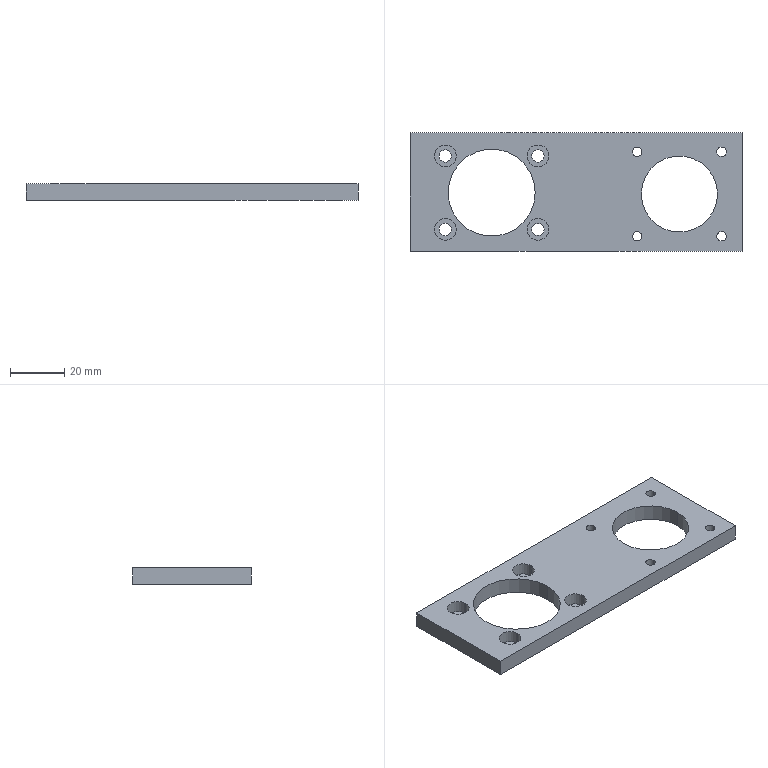Part | SolidWorks | features BaseBody 1 | 1 solid | 38 faces | box 122 x 43.5 x 6 mm | volume 22091 mm3 | cylinder 28 | plane 10 | commonest cylinder face diameters 3.5 x8 4.5 x8 8 x8 28 x2 32 x2
STEP:
#1=CARTESIAN_POINT('',(83.24,-0.6873,6.));
#2=VERTEX_POINT('',#1);
#3=CARTESIAN_POINT('',(55.24,-0.6873,6.));
#4=VERTEX_POINT('',#3);
#5=CARTESIAN_POINT('',(69.24,-0.6873,6.));
#6=DIRECTION('',(0.,0.,-1.));
#7=DIRECTION('',(-1.,0.,0.));
#8=AXIS2_PLACEMENT_3D('',#5,#6,#7);
#9=CIRCLE('',#8,14.);
#10=EDGE_CURVE('',#2,#4,#9,.T.);
#11=ORIENTED_EDGE('',*,*,#10,.F.);
#12=CARTESIAN_POINT('',(83.24,-0.6873,0.));
#13=VERTEX_POINT('',#12);
#14=CARTESIAN_POINT('',(83.24,-0.6873,6.));
#15=DIRECTION('',(0.,0.,-1.));
#16=VECTOR('',#15,1000.);
#17=LINE('',#14,#16);
#18=EDGE_CURVE('',#2,#13,#17,.T.);
#19=ORIENTED_EDGE('',*,*,#18,.T.);
#20=CARTESIAN_POINT('',(55.24,-0.6873,0.));
#21=VERTEX_POINT('',#20);
#22=CARTESIAN_POINT('',(69.24,-0.6873,0.));
#23=DIRECTION('',(0.,0.,-1.));
#24=DIRECTION('',(-1.,0.,0.));
#25=AXIS2_PLACEMENT_3D('',#22,#23,#24);
#26=CIRCLE('',#25,14.);
#27=EDGE_CURVE('',#13,#21,#26,.T.);
#28=ORIENTED_EDGE('',*,*,#27,.T.);
#29=CARTESIAN_POINT('',(55.24,-0.6873,6.));
#30=DIRECTION('',(0.,0.,-1.));
#31=VECTOR('',#30,1000.);
#32=LINE('',#29,#31);
#33=EDGE_CURVE('',#4,#21,#32,.T.);
#34=ORIENTED_EDGE('',*,*,#33,.F.);
#35=EDGE_LOOP('',(#11,#19,#28,#34));
#36=FACE_OUTER_BOUND('',#35,.T.);
#37=CARTESIAN_POINT('',(69.24,-0.6873,6.));
#38=DIRECTION('',(0.,0.,-1.));
#39=DIRECTION('',(-1.,0.,0.));
#40=AXIS2_PLACEMENT_3D('',#37,#38,#39);
#41=CYLINDRICAL_SURFACE('',#40,14.);
#42=ADVANCED_FACE('',(#36),#41,.F.);
#43=CARTESIAN_POINT('',(16.24,-0.1873,6.));
#44=VERTEX_POINT('',#43);
#45=CARTESIAN_POINT('',(-15.76,-0.1873,6.));
#46=VERTEX_POINT('',#45);
#47=CARTESIAN_POINT('',(0.2397,-0.1873,6.));
#48=DIRECTION('',(0.,0.,-1.));
#49=DIRECTION('',(-1.,0.,0.));
#50=AXIS2_PLACEMENT_3D('',#47,#48,#49);
#51=CIRCLE('',#50,16.);
#52=EDGE_CURVE('',#44,#46,#51,.T.);
#53=ORIENTED_EDGE('',*,*,#52,.F.);
#54=CARTESIAN_POINT('',(16.24,-0.1873,0.));
#55=VERTEX_POINT('',#54);
#56=CARTESIAN_POINT('',(16.24,-0.1873,6.));
#57=DIRECTION('',(0.,0.,-1.));
#58=VECTOR('',#57,1000.);
#59=LINE('',#56,#58);
#60=EDGE_CURVE('',#44,#55,#59,.T.);
#61=ORIENTED_EDGE('',*,*,#60,.T.);
#62=CARTESIAN_POINT('',(-15.76,-0.1873,0.));
#63=VERTEX_POINT('',#62);
#64=CARTESIAN_POINT('',(0.2397,-0.1873,0.));
#65=DIRECTION('',(0.,0.,-1.));
#66=DIRECTION('',(-1.,0.,0.));
#67=AXIS2_PLACEMENT_3D('',#64,#65,#66);
#68=CIRCLE('',#67,16.);
#69=EDGE_CURVE('',#55,#63,#68,.T.);
#70=ORIENTED_EDGE('',*,*,#69,.T.);
#71=CARTESIAN_POINT('',(-15.76,-0.1873,6.));
#72=DIRECTION('',(0.,0.,-1.));
#73=VECTOR('',#72,1000.);
#74=LINE('',#71,#73);
#75=EDGE_CURVE('',#46,#63,#74,.T.);
#76=ORIENTED_EDGE('',*,*,#75,.F.);
#77=EDGE_LOOP('',(#53,#61,#70,#76));
#78=FACE_OUTER_BOUND('',#77,.T.);
#79=CARTESIAN_POINT('',(0.2397,-0.1873,6.));
#80=DIRECTION('',(0.,0.,-1.));
#81=DIRECTION('',(-1.,0.,0.));
#82=AXIS2_PLACEMENT_3D('',#79,#80,#81);
#83=CYLINDRICAL_SURFACE('',#82,16.);
#84=ADVANCED_FACE('',(#78),#83,.F.);
#85=CARTESIAN_POINT('',(55.49,14.813,0.));
#86=VERTEX_POINT('',#85);
#87=CARTESIAN_POINT('',(51.99,14.813,0.));
#88=VERTEX_POINT('',#87);
#89=CARTESIAN_POINT('',(53.74,14.813,0.));
#90=DIRECTION('',(0.,0.,-1.));
#91=DIRECTION('',(1.,0.,0.));
#92=AXIS2_PLACEMENT_3D('',#89,#90,#91);
#93=CIRCLE('',#92,1.75);
#94=EDGE_CURVE('',#86,#88,#93,.T.);
#95=ORIENTED_EDGE('',*,*,#94,.T.);
#96=CARTESIAN_POINT('',(51.99,14.813,6.));
#97=VERTEX_POINT('',#96);
#98=CARTESIAN_POINT('',(51.99,14.813,-123.662));
#99=DIRECTION('',(0.,0.,1.));
#100=VECTOR('',#99,1000.);
#101=LINE('',#98,#100);
#102=EDGE_CURVE('',#88,#97,#101,.T.);
#103=ORIENTED_EDGE('',*,*,#102,.T.);
#104=CARTESIAN_POINT('',(55.49,14.813,6.));
#105=VERTEX_POINT('',#104);
#106=CARTESIAN_POINT('',(53.74,14.813,6.));
#107=DIRECTION('',(0.,0.,-1.));
#108=DIRECTION('',(1.,0.,0.));
#109=AXIS2_PLACEMENT_3D('',#106,#107,#108);
#110=CIRCLE('',#109,1.75);
#111=EDGE_CURVE('',#105,#97,#110,.T.);
#112=ORIENTED_EDGE('',*,*,#111,.F.);
#113=CARTESIAN_POINT('',(55.49,14.813,-123.662));
#114=DIRECTION('',(0.,0.,1.));
#115=VECTOR('',#114,1000.);
#116=LINE('',#113,#115);
#117=EDGE_CURVE('',#86,#105,#116,.T.);
#118=ORIENTED_EDGE('',*,*,#117,.F.);
#119=EDGE_LOOP('',(#95,#103,#112,#118));
#120=FACE_OUTER_BOUND('',#119,.T.);
#121=CARTESIAN_POINT('',(53.74,14.813,-123.662));
#122=DIRECTION('',(0.,0.,1.));
#123=DIRECTION('',(1.,0.,0.));
#124=AXIS2_PLACEMENT_3D('',#121,#122,#123);
#125=CYLINDRICAL_SURFACE('',#124,1.75);
#126=ADVANCED_FACE('',(#120),#125,.F.);
#127=CARTESIAN_POINT('',(86.49,14.813,0.));
#128=VERTEX_POINT('',#127);
#129=CARTESIAN_POINT('',(82.99,14.813,0.));
#130=VERTEX_POINT('',#129);
#131=CARTESIAN_POINT('',(84.74,14.813,0.));
#132=DIRECTION('',(0.,0.,-1.));
#133=DIRECTION('',(1.,0.,0.));
#134=AXIS2_PLACEMENT_3D('',#131,#132,#133);
#135=CIRCLE('',#134,1.75);
#136=EDGE_CURVE('',#128,#130,#135,.T.);
#137=ORIENTED_EDGE('',*,*,#136,.T.);
#138=CARTESIAN_POINT('',(82.99,14.813,6.));
#139=VERTEX_POINT('',#138);
#140=CARTESIAN_POINT('',(82.99,14.813,-123.662));
#141=DIRECTION('',(0.,0.,1.));
#142=VECTOR('',#141,1000.);
#143=LINE('',#140,#142);
#144=EDGE_CURVE('',#130,#139,#143,.T.);
#145=ORIENTED_EDGE('',*,*,#144,.T.);
#146=CARTESIAN_POINT('',(86.49,14.813,6.));
#147=VERTEX_POINT('',#146);
#148=CARTESIAN_POINT('',(84.74,14.813,6.));
#149=DIRECTION('',(0.,0.,-1.));
#150=DIRECTION('',(1.,0.,0.));
#151=AXIS2_PLACEMENT_3D('',#148,#149,#150);
#152=CIRCLE('',#151,1.75);
#153=EDGE_CURVE('',#147,#139,#152,.T.);
#154=ORIENTED_EDGE('',*,*,#153,.F.);
#155=CARTESIAN_POINT('',(86.49,14.813,-123.662));
#156=DIRECTION('',(0.,0.,1.));
#157=VECTOR('',#156,1000.);
#158=LINE('',#155,#157);
#159=EDGE_CURVE('',#128,#147,#158,.T.);
#160=ORIENTED_EDGE('',*,*,#159,.F.);
#161=EDGE_LOOP('',(#137,#145,#154,#160));
#162=FACE_OUTER_BOUND('',#161,.T.);
#163=CARTESIAN_POINT('',(84.74,14.813,-123.662));
#164=DIRECTION('',(0.,0.,1.));
#165=DIRECTION('',(1.,0.,0.));
#166=AXIS2_PLACEMENT_3D('',#163,#164,#165);
#167=CYLINDRICAL_SURFACE('',#166,1.75);
#168=ADVANCED_FACE('',(#162),#167,.F.);
#169=CARTESIAN_POINT('',(86.49,-16.187,0.));
#170=VERTEX_POINT('',#169);
#171=CARTESIAN_POINT('',(82.99,-16.187,0.));
#172=VERTEX_POINT('',#171);
#173=CARTESIAN_POINT('',(84.74,-16.187,0.));
#174=DIRECTION('',(0.,0.,-1.));
#175=DIRECTION('',(1.,0.,0.));
#176=AXIS2_PLACEMENT_3D('',#173,#174,#175);
#177=CIRCLE('',#176,1.75);
#178=EDGE_CURVE('',#170,#172,#177,.T.);
#179=ORIENTED_EDGE('',*,*,#178,.T.);
#180=CARTESIAN_POINT('',(82.99,-16.187,6.));
#181=VERTEX_POINT('',#180);
#182=CARTESIAN_POINT('',(82.99,-16.187,-123.662));
#183=DIRECTION('',(0.,0.,1.));
#184=VECTOR('',#183,1000.);
#185=LINE('',#182,#184);
#186=EDGE_CURVE('',#172,#181,#185,.T.);
#187=ORIENTED_EDGE('',*,*,#186,.T.);
#188=CARTESIAN_POINT('',(86.49,-16.187,6.));
#189=VERTEX_POINT('',#188);
#190=CARTESIAN_POINT('',(84.74,-16.187,6.));
#191=DIRECTION('',(0.,0.,-1.));
#192=DIRECTION('',(1.,0.,0.));
#193=AXIS2_PLACEMENT_3D('',#190,#191,#192);
#194=CIRCLE('',#193,1.75);
#195=EDGE_CURVE('',#189,#181,#194,.T.);
#196=ORIENTED_EDGE('',*,*,#195,.F.);
#197=CARTESIAN_POINT('',(86.49,-16.187,-123.662));
#198=DIRECTION('',(0.,0.,1.));
#199=VECTOR('',#198,1000.);
#200=LINE('',#197,#199);
#201=EDGE_CURVE('',#170,#189,#200,.T.);
#202=ORIENTED_EDGE('',*,*,#201,.F.);
#203=EDGE_LOOP('',(#179,#187,#196,#202));
#204=FACE_OUTER_BOUND('',#203,.T.);
#205=CARTESIAN_POINT('',(84.74,-16.187,-123.662));
#206=DIRECTION('',(0.,0.,1.));
#207=DIRECTION('',(1.,0.,0.));
#208=AXIS2_PLACEMENT_3D('',#205,#206,#207);
#209=CYLINDRICAL_SURFACE('',#208,1.75);
#210=ADVANCED_FACE('',(#204),#209,.F.);
#211=CARTESIAN_POINT('',(55.49,-16.187,0.));
#212=VERTEX_POINT('',#211);
#213=CARTESIAN_POINT('',(51.99,-16.187,0.));
#214=VERTEX_POINT('',#213);
#215=CARTESIAN_POINT('',(53.74,-16.187,0.));
#216=DIRECTION('',(0.,0.,-1.));
#217=DIRECTION('',(1.,0.,0.));
#218=AXIS2_PLACEMENT_3D('',#215,#216,#217);
#219=CIRCLE('',#218,1.75);
#220=EDGE_CURVE('',#212,#214,#219,.T.);
#221=ORIENTED_EDGE('',*,*,#220,.T.);
#222=CARTESIAN_POINT('',(51.99,-16.187,6.));
#223=VERTEX_POINT('',#222);
#224=CARTESIAN_POINT('',(51.99,-16.187,-123.662));
#225=DIRECTION('',(0.,0.,1.));
#226=VECTOR('',#225,1000.);
#227=LINE('',#224,#226);
#228=EDGE_CURVE('',#214,#223,#227,.T.);
#229=ORIENTED_EDGE('',*,*,#228,.T.);
#230=CARTESIAN_POINT('',(55.49,-16.187,6.));
#231=VERTEX_POINT('',#230);
#232=CARTESIAN_POINT('',(53.74,-16.187,6.));
#233=DIRECTION('',(0.,0.,-1.));
#234=DIRECTION('',(1.,0.,0.));
#235=AXIS2_PLACEMENT_3D('',#232,#233,#234);
#236=CIRCLE('',#235,1.75);
#237=EDGE_CURVE('',#231,#223,#236,.T.);
#238=ORIENTED_EDGE('',*,*,#237,.F.);
#239=CARTESIAN_POINT('',(55.49,-16.187,-123.662));
#240=DIRECTION('',(0.,0.,1.));
#241=VECTOR('',#240,1000.);
#242=LINE('',#239,#241);
#243=EDGE_CURVE('',#212,#231,#242,.T.);
#244=ORIENTED_EDGE('',*,*,#243,.F.);
#245=EDGE_LOOP('',(#221,#229,#238,#244));
#246=FACE_OUTER_BOUND('',#245,.T.);
#247=CARTESIAN_POINT('',(53.74,-16.187,-123.662));
#248=DIRECTION('',(0.,0.,1.));
#249=DIRECTION('',(1.,0.,0.));
#250=AXIS2_PLACEMENT_3D('',#247,#248,#249);
#251=CYLINDRICAL_SURFACE('',#250,1.75);
#252=ADVANCED_FACE('',(#246),#251,.F.);
#253=CARTESIAN_POINT('',(-14.51,13.313,0.));
#254=VERTEX_POINT('',#253);
#255=CARTESIAN_POINT('',(-19.01,13.313,0.));
#256=VERTEX_POINT('',#255);
#257=CARTESIAN_POINT('',(-16.76,13.313,0.));
#258=DIRECTION('',(0.,0.,-1.));
#259=DIRECTION('',(1.,0.,0.));
#260=AXIS2_PLACEMENT_3D('',#257,#258,#259);
#261=CIRCLE('',#260,2.25);
#262=EDGE_CURVE('',#254,#256,#261,.T.);
#263=ORIENTED_EDGE('',*,*,#262,.T.);
#264=CARTESIAN_POINT('',(-19.01,13.313,1.5));
#265=VERTEX_POINT('',#264);
#266=CARTESIAN_POINT('',(-19.01,13.313,-123.662));
#267=DIRECTION('',(0.,0.,1.));
#268=VECTOR('',#267,1000.);
#269=LINE('',#266,#268);
#270=EDGE_CURVE('',#256,#265,#269,.T.);
#271=ORIENTED_EDGE('',*,*,#270,.T.);
#272=CARTESIAN_POINT('',(-14.51,13.313,1.5));
#273=VERTEX_POINT('',#272);
#274=CARTESIAN_POINT('',(-16.76,13.313,1.5));
#275=DIRECTION('',(0.,0.,-1.));
#276=DIRECTION('',(1.,0.,0.));
#277=AXIS2_PLACEMENT_3D('',#274,#275,#276);
#278=CIRCLE('',#277,2.25);
#279=EDGE_CURVE('',#273,#265,#278,.T.);
#280=ORIENTED_EDGE('',*,*,#279,.F.);
#281=CARTESIAN_POINT('',(-14.51,13.313,-123.662));
#282=DIRECTION('',(0.,0.,1.));
#283=VECTOR('',#282,1000.);
#284=LINE('',#281,#283);
#285=EDGE_CURVE('',#254,#273,#284,.T.);
#286=ORIENTED_EDGE('',*,*,#285,.F.);
#287=EDGE_LOOP('',(#263,#271,#280,#286));
#288=FACE_OUTER_BOUND('',#287,.T.);
#289=CARTESIAN_POINT('',(-16.76,13.313,-123.662));
#290=DIRECTION('',(0.,0.,1.));
#291=DIRECTION('',(1.,0.,0.));
#292=AXIS2_PLACEMENT_3D('',#289,#290,#291);
#293=CYLINDRICAL_SURFACE('',#292,2.25);
#294=ADVANCED_FACE('',(#288),#293,.F.);
#295=CARTESIAN_POINT('',(19.49,13.313,0.));
#296=VERTEX_POINT('',#295);
#297=CARTESIAN_POINT('',(14.99,13.313,0.));
#298=VERTEX_POINT('',#297);
#299=CARTESIAN_POINT('',(17.24,13.313,0.));
#300=DIRECTION('',(0.,0.,-1.));
#301=DIRECTION('',(1.,0.,0.));
#302=AXIS2_PLACEMENT_3D('',#299,#300,#301);
#303=CIRCLE('',#302,2.25);
#304=EDGE_CURVE('',#296,#298,#303,.T.);
#305=ORIENTED_EDGE('',*,*,#304,.T.);
#306=CARTESIAN_POINT('',(14.99,13.313,1.5));
#307=VERTEX_POINT('',#306);
#308=CARTESIAN_POINT('',(14.99,13.313,-123.662));
#309=DIRECTION('',(0.,0.,1.));
#310=VECTOR('',#309,1000.);
#311=LINE('',#308,#310);
#312=EDGE_CURVE('',#298,#307,#311,.T.);
#313=ORIENTED_EDGE('',*,*,#312,.T.);
#314=CARTESIAN_POINT('',(19.49,13.313,1.5));
#315=VERTEX_POINT('',#314);
#316=CARTESIAN_POINT('',(17.24,13.313,1.5));
#317=DIRECTION('',(0.,0.,-1.));
#318=DIRECTION('',(1.,0.,0.));
#319=AXIS2_PLACEMENT_3D('',#316,#317,#318);
#320=CIRCLE('',#319,2.25);
#321=EDGE_CURVE('',#315,#307,#320,.T.);
#322=ORIENTED_EDGE('',*,*,#321,.F.);
#323=CARTESIAN_POINT('',(19.49,13.313,-123.662));
#324=DIRECTION('',(0.,0.,1.));
#325=VECTOR('',#324,1000.);
#326=LINE('',#323,#325);
#327=EDGE_CURVE('',#296,#315,#326,.T.);
#328=ORIENTED_EDGE('',*,*,#327,.F.);
#329=EDGE_LOOP('',(#305,#313,#322,#328));
#330=FACE_OUTER_BOUND('',#329,.T.);
#331=CARTESIAN_POINT('',(17.24,13.313,-123.662));
#332=DIRECTION('',(0.,0.,1.));
#333=DIRECTION('',(1.,0.,0.));
#334=AXIS2_PLACEMENT_3D('',#331,#332,#333);
#335=CYLINDRICAL_SURFACE('',#334,2.25);
#336=ADVANCED_FACE('',(#330),#335,.F.);
#337=CARTESIAN_POINT('',(-14.51,-13.687,0.));
#338=VERTEX_POINT('',#337);
#339=CARTESIAN_POINT('',(-19.01,-13.687,0.));
#340=VERTEX_POINT('',#339);
#341=CARTESIAN_POINT('',(-16.76,-13.687,0.));
#342=DIRECTION('',(0.,0.,-1.));
#343=DIRECTION('',(1.,0.,0.));
#344=AXIS2_PLACEMENT_3D('',#341,#342,#343);
#345=CIRCLE('',#344,2.25);
#346=EDGE_CURVE('',#338,#340,#345,.T.);
#347=ORIENTED_EDGE('',*,*,#346,.T.);
#348=CARTESIAN_POINT('',(-19.01,-13.687,1.5));
#349=VERTEX_POINT('',#348);
#350=CARTESIAN_POINT('',(-19.01,-13.687,-123.662));
#351=DIRECTION('',(0.,0.,1.));
#352=VECTOR('',#351,1000.);
#353=LINE('',#350,#352);
#354=EDGE_CURVE('',#340,#349,#353,.T.);
#355=ORIENTED_EDGE('',*,*,#354,.T.);
#356=CARTESIAN_POINT('',(-14.51,-13.687,1.5));
#357=VERTEX_POINT('',#356);
#358=CARTESIAN_POINT('',(-16.76,-13.687,1.5));
#359=DIRECTION('',(0.,0.,-1.));
#360=DIRECTION('',(1.,0.,0.));
#361=AXIS2_PLACEMENT_3D('',#358,#359,#360);
#362=CIRCLE('',#361,2.25);
#363=EDGE_CURVE('',#357,#349,#362,.T.);
#364=ORIENTED_EDGE('',*,*,#363,.F.);
#365=CARTESIAN_POINT('',(-14.51,-13.687,-123.662));
#366=DIRECTION('',(0.,0.,1.));
#367=VECTOR('',#366,1000.);
#368=LINE('',#365,#367);
#369=EDGE_CURVE('',#338,#357,#368,.T.);
#370=ORIENTED_EDGE('',*,*,#369,.F.);
#371=EDGE_LOOP('',(#347,#355,#364,#370));
#372=FACE_OUTER_BOUND('',#371,.T.);
#373=CARTESIAN_POINT('',(-16.76,-13.687,-123.662));
#374=DIRECTION('',(0.,0.,1.));
#375=DIRECTION('',(1.,0.,0.));
#376=AXIS2_PLACEMENT_3D('',#373,#374,#375);
#377=CYLINDRICAL_SURFACE('',#376,2.25);
#378=ADVANCED_FACE('',(#372),#377,.F.);
#379=CARTESIAN_POINT('',(19.49,-13.687,0.));
#380=VERTEX_POINT('',#379);
#381=CARTESIAN_POINT('',(14.99,-13.687,0.));
#382=VERTEX_POINT('',#381);
#383=CARTESIAN_POINT('',(17.24,-13.687,0.));
#384=DIRECTION('',(0.,0.,-1.));
#385=DIRECTION('',(1.,0.,0.));
#386=AXIS2_PLACEMENT_3D('',#383,#384,#385);
#387=CIRCLE('',#386,2.25);
#388=EDGE_CURVE('',#380,#382,#387,.T.);
#389=ORIENTED_EDGE('',*,*,#388,.T.);
#390=CARTESIAN_POINT('',(14.99,-13.687,1.5));
#391=VERTEX_POINT('',#390);
#392=CARTESIAN_POINT('',(14.99,-13.687,-123.662));
#393=DIRECTION('',(0.,0.,1.));
#394=VECTOR('',#393,1000.);
#395=LINE('',#392,#394);
#396=EDGE_CURVE('',#382,#391,#395,.T.);
#397=ORIENTED_EDGE('',*,*,#396,.T.);
#398=CARTESIAN_POINT('',(19.49,-13.687,1.5));
#399=VERTEX_POINT('',#398);
#400=CARTESIAN_POINT('',(17.24,-13.687,1.5));
#401=DIRECTION('',(0.,0.,-1.));
#402=DIRECTION('',(1.,0.,0.));
#403=AXIS2_PLACEMENT_3D('',#400,#401,#402);
#404=CIRCLE('',#403,2.25);
#405=EDGE_CURVE('',#399,#391,#404,.T.);
#406=ORIENTED_EDGE('',*,*,#405,.F.);
#407=CARTESIAN_POINT('',(19.49,-13.687,-123.662));
#408=DIRECTION('',(0.,0.,1.));
#409=VECTOR('',#408,1000.);
#410=LINE('',#407,#409);
#411=EDGE_CURVE('',#380,#399,#410,.T.);
#412=ORIENTED_EDGE('',*,*,#411,.F.);
#413=EDGE_LOOP('',(#389,#397,#406,#412));
#414=FACE_OUTER_BOUND('',#413,.T.);
#415=CARTESIAN_POINT('',(17.24,-13.687,-123.662));
#416=DIRECTION('',(0.,0.,1.));
#417=DIRECTION('',(1.,0.,0.));
#418=AXIS2_PLACEMENT_3D('',#415,#416,#417);
#419=CYLINDRICAL_SURFACE('',#418,2.25);
#420=ADVANCED_FACE('',(#414),#419,.F.);
#421=CARTESIAN_POINT('',(-20.76,13.313,1.5));
#422=VERTEX_POINT('',#421);
#423=CARTESIAN_POINT('',(-12.76,13.313,1.5));
#424=VERTEX_POINT('',#423);
#425=CARTESIAN_POINT('',(-16.76,13.313,1.5));
#426=DIRECTION('',(0.,0.,1.));
#427=DIRECTION('',(1.,0.,0.));
#428=AXIS2_PLACEMENT_3D('',#425,#426,#427);
#429=CIRCLE('',#428,4.);
#430=EDGE_CURVE('',#422,#424,#429,.T.);
#431=ORIENTED_EDGE('',*,*,#430,.F.);
#432=CARTESIAN_POINT('',(-20.76,13.313,6.));
#433=VERTEX_POINT('',#432);
#434=CARTESIAN_POINT('',(-20.76,13.313,3.75));
#435=DIRECTION('',(0.,0.,1.));
#436=VECTOR('',#435,1000.);
#437=LINE('',#434,#436);
#438=EDGE_CURVE('',#422,#433,#437,.T.);
#439=ORIENTED_EDGE('',*,*,#438,.T.);
#440=CARTESIAN_POINT('',(-12.76,13.313,6.));
#441=VERTEX_POINT('',#440);
#442=CARTESIAN_POINT('',(-16.76,13.313,6.));
#443=DIRECTION('',(0.,0.,-1.));
#444=DIRECTION('',(1.,0.,0.));
#445=AXIS2_PLACEMENT_3D('',#442,#443,#444);
#446=CIRCLE('',#445,4.);
#447=EDGE_CURVE('',#441,#433,#446,.T.);
#448=ORIENTED_EDGE('',*,*,#447,.F.);
#449=CARTESIAN_POINT('',(-12.76,13.313,3.75));
#450=DIRECTION('',(0.,0.,1.));
#451=VECTOR('',#450,1000.);
#452=LINE('',#449,#451);
#453=EDGE_CURVE('',#424,#441,#452,.T.);
#454=ORIENTED_EDGE('',*,*,#453,.F.);
#455=EDGE_LOOP('',(#431,#439,#448,#454));
#456=FACE_OUTER_BOUND('',#455,.T.);
#457=CARTESIAN_POINT('',(-16.76,13.313,3.75));
#458=DIRECTION('',(0.,0.,1.));
#459=DIRECTION('',(1.,0.,0.));
#460=AXIS2_PLACEMENT_3D('',#457,#458,#459);
#461=CYLINDRICAL_SURFACE('',#460,4.);
#462=ADVANCED_FACE('',(#456),#461,.F.);
#463=CARTESIAN_POINT('',(13.24,13.313,1.5));
#464=VERTEX_POINT('',#463);
#465=CARTESIAN_POINT('',(21.24,13.313,1.5));
#466=VERTEX_POINT('',#465);
#467=CARTESIAN_POINT('',(17.24,13.313,1.5));
#468=DIRECTION('',(0.,0.,1.));
#469=DIRECTION('',(1.,0.,0.));
#470=AXIS2_PLACEMENT_3D('',#467,#468,#469);
#471=CIRCLE('',#470,4.);
#472=EDGE_CURVE('',#464,#466,#471,.T.);
#473=ORIENTED_EDGE('',*,*,#472,.F.);
#474=CARTESIAN_POINT('',(13.24,13.313,6.));
#475=VERTEX_POINT('',#474);
#476=CARTESIAN_POINT('',(13.24,13.313,3.75));
#477=DIRECTION('',(0.,0.,1.));
#478=VECTOR('',#477,1000.);
#479=LINE('',#476,#478);
#480=EDGE_CURVE('',#464,#475,#479,.T.);
#481=ORIENTED_EDGE('',*,*,#480,.T.);
#482=CARTESIAN_POINT('',(21.24,13.313,6.));
#483=VERTEX_POINT('',#482);
#484=CARTESIAN_POINT('',(17.24,13.313,6.));
#485=DIRECTION('',(0.,0.,-1.));
#486=DIRECTION('',(1.,0.,0.));
#487=AXIS2_PLACEMENT_3D('',#484,#485,#486);
#488=CIRCLE('',#487,4.);
#489=EDGE_CURVE('',#483,#475,#488,.T.);
#490=ORIENTED_EDGE('',*,*,#489,.F.);
#491=CARTESIAN_POINT('',(21.24,13.313,3.75));
#492=DIRECTION('',(0.,0.,1.));
#493=VECTOR('',#492,1000.);
#494=LINE('',#491,#493);
#495=EDGE_CURVE('',#466,#483,#494,.T.);
#496=ORIENTED_EDGE('',*,*,#495,.F.);
#497=EDGE_LOOP('',(#473,#481,#490,#496));
#498=FACE_OUTER_BOUND('',#497,.T.);
#499=CARTESIAN_POINT('',(17.24,13.313,3.75));
#500=DIRECTION('',(0.,0.,1.));
#501=DIRECTION('',(1.,0.,0.));
#502=AXIS2_PLACEMENT_3D('',#499,#500,#501);
#503=CYLINDRICAL_SURFACE('',#502,4.);
#504=ADVANCED_FACE('',(#498),#503,.F.);
#505=CARTESIAN_POINT('',(-20.76,-13.687,1.5));
#506=VERTEX_POINT('',#505);
#507=CARTESIAN_POINT('',(-12.76,-13.687,1.5));
#508=VERTEX_POINT('',#507);
#509=CARTESIAN_POINT('',(-16.76,-13.687,1.5));
#510=DIRECTION('',(0.,0.,1.));
#511=DIRECTION('',(1.,0.,0.));
#512=AXIS2_PLACEMENT_3D('',#509,#510,#511);
#513=CIRCLE('',#512,4.);
#514=EDGE_CURVE('',#506,#508,#513,.T.);
#515=ORIENTED_EDGE('',*,*,#514,.F.);
#516=CARTESIAN_POINT('',(-20.76,-13.687,6.));
#517=VERTEX_POINT('',#516);
#518=CARTESIAN_POINT('',(-20.76,-13.687,3.75));
#519=DIRECTION('',(0.,0.,1.));
#520=VECTOR('',#519,1000.);
#521=LINE('',#518,#520);
#522=EDGE_CURVE('',#506,#517,#521,.T.);
#523=ORIENTED_EDGE('',*,*,#522,.T.);
#524=CARTESIAN_POINT('',(-12.76,-13.687,6.));
#525=VERTEX_POINT('',#524);
#526=CARTESIAN_POINT('',(-16.76,-13.687,6.));
#527=DIRECTION('',(0.,0.,-1.));
#528=DIRECTION('',(1.,0.,0.));
#529=AXIS2_PLACEMENT_3D('',#526,#527,#528);
#530=CIRCLE('',#529,4.);
#531=EDGE_CURVE('',#525,#517,#530,.T.);
#532=ORIENTED_EDGE('',*,*,#531,.F.);
#533=CARTESIAN_POINT('',(-12.76,-13.687,3.75));
#534=DIRECTION('',(0.,0.,1.));
#535=VECTOR('',#534,1000.);
#536=LINE('',#533,#535);
#537=EDGE_CURVE('',#508,#525,#536,.T.);
#538=ORIENTED_EDGE('',*,*,#537,.F.);
#539=EDGE_LOOP('',(#515,#523,#532,#538));
#540=FACE_OUTER_BOUND('',#539,.T.);
#541=CARTESIAN_POINT('',(-16.76,-13.687,3.75));
#542=DIRECTION('',(0.,0.,1.));
#543=DIRECTION('',(1.,0.,0.));
#544=AXIS2_PLACEMENT_3D('',#541,#542,#543);
#545=CYLINDRICAL_SURFACE('',#544,4.);
#546=ADVANCED_FACE('',(#540),#545,.F.);
#547=CARTESIAN_POINT('',(13.24,-13.687,1.5));
#548=VERTEX_POINT('',#547);
#549=CARTESIAN_POINT('',(21.24,-13.687,1.5));
#550=VERTEX_POINT('',#549);
#551=CARTESIAN_POINT('',(17.24,-13.687,1.5));
#552=DIRECTION('',(0.,0.,1.));
#553=DIRECTION('',(1.,0.,0.));
#554=AXIS2_PLACEMENT_3D('',#551,#552,#553);
#555=CIRCLE('',#554,4.);
#556=EDGE_CURVE('',#548,#550,#555,.T.);
#557=ORIENTED_EDGE('',*,*,#556,.F.);
#558=CARTESIAN_POINT('',(13.24,-13.687,6.));
#559=VERTEX_POINT('',#558);
#560=CARTESIAN_POINT('',(13.24,-13.687,3.75));
#561=DIRECTION('',(0.,0.,1.));
#562=VECTOR('',#561,1000.);
#563=LINE('',#560,#562);
#564=EDGE_CURVE('',#548,#559,#563,.T.);
#565=ORIENTED_EDGE('',*,*,#564,.T.);
#566=CARTESIAN_POINT('',(21.24,-13.687,6.));
#567=VERTEX_POINT('',#566);
#568=CARTESIAN_POINT('',(17.24,-13.687,6.));
#569=DIRECTION('',(0.,0.,-1.));
#570=DIRECTION('',(1.,0.,0.));
#571=AXIS2_PLACEMENT_3D('',#568,#569,#570);
#572=CIRCLE('',#571,4.);
#573=EDGE_CURVE('',#567,#559,#572,.T.);
#574=ORIENTED_EDGE('',*,*,#573,.F.);
#575=CARTESIAN_POINT('',(21.24,-13.687,3.75));
#576=DIRECTION('',(0.,0.,1.));
#577=VECTOR('',#576,1000.);
#578=LINE('',#575,#577);
#579=EDGE_CURVE('',#550,#567,#578,.T.);
#580=ORIENTED_EDGE('',*,*,#579,.F.);
#581=EDGE_LOOP('',(#557,#565,#574,#580));
#582=FACE_OUTER_BOUND('',#581,.T.);
#583=CARTESIAN_POINT('',(17.24,-13.687,3.75));
#584=DIRECTION('',(0.,0.,1.));
#585=DIRECTION('',(1.,0.,0.));
#586=AXIS2_PLACEMENT_3D('',#583,#584,#585);
#587=CYLINDRICAL_SURFACE('',#586,4.);
#588=ADVANCED_FACE('',(#582),#587,.F.);
#589=CARTESIAN_POINT('',(69.24,-0.6873,0.));
#590=DIRECTION('',(0.,0.,-1.));
#591=DIRECTION('',(-1.,0.,0.));
#592=AXIS2_PLACEMENT_3D('',#589,#590,#591);
#593=CIRCLE('',#592,14.);
#594=EDGE_CURVE('',#21,#13,#593,.T.);
#595=ORIENTED_EDGE('',*,*,#594,.F.);
#596=ORIENTED_EDGE('',*,*,#27,.F.);
#597=EDGE_LOOP('',(#595,#596));
#598=FACE_BOUND('',#597,.T.);
#599=CARTESIAN_POINT('',(0.2397,-0.1873,0.));
#600=DIRECTION('',(0.,0.,-1.));
#601=DIRECTION('',(-1.,0.,0.));
#602=AXIS2_PLACEMENT_3D('',#599,#600,#601);
#603=CIRCLE('',#602,16.);
#604=EDGE_CURVE('',#63,#55,#603,.T.);
#605=ORIENTED_EDGE('',*,*,#604,.F.);
#606=ORIENTED_EDGE('',*,*,#69,.F.);
#607=EDGE_LOOP('',(#605,#606));
#608=FACE_BOUND('',#607,.T.);
#609=ORIENTED_EDGE('',*,*,#94,.F.);
#610=CARTESIAN_POINT('',(53.74,14.813,0.));
#611=DIRECTION('',(0.,0.,-1.));
#612=DIRECTION('',(1.,0.,0.));
#613=AXIS2_PLACEMENT_3D('',#610,#611,#612);
#614=CIRCLE('',#613,1.75);
#615=EDGE_CURVE('',#88,#86,#614,.T.);
#616=ORIENTED_EDGE('',*,*,#615,.F.);
#617=EDGE_LOOP('',(#609,#616));
#618=FACE_BOUND('',#617,.T.);
#619=ORIENTED_EDGE('',*,*,#136,.F.);
#620=CARTESIAN_POINT('',(84.74,14.813,0.));
#621=DIRECTION('',(0.,0.,-1.));
#622=DIRECTION('',(1.,0.,0.));
#623=AXIS2_PLACEMENT_3D('',#620,#621,#622);
#624=CIRCLE('',#623,1.75);
#625=EDGE_CURVE('',#130,#128,#624,.T.);
#626=ORIENTED_EDGE('',*,*,#625,.F.);
#627=EDGE_LOOP('',(#619,#626));
#628=FACE_BOUND('',#627,.T.);
#629=ORIENTED_EDGE('',*,*,#178,.F.);
#630=CARTESIAN_POINT('',(84.74,-16.187,0.));
#631=DIRECTION('',(0.,0.,-1.));
#632=DIRECTION('',(1.,0.,0.));
#633=AXIS2_PLACEMENT_3D('',#630,#631,#632);
#634=CIRCLE('',#633,1.75);
#635=EDGE_CURVE('',#172,#170,#634,.T.);
#636=ORIENTED_EDGE('',*,*,#635,.F.);
#637=EDGE_LOOP('',(#629,#636));
#638=FACE_BOUND('',#637,.T.);
#639=ORIENTED_EDGE('',*,*,#220,.F.);
#640=CARTESIAN_POINT('',(53.74,-16.187,0.));
#641=DIRECTION('',(0.,0.,-1.));
#642=DIRECTION('',(1.,0.,0.));
#643=AXIS2_PLACEMENT_3D('',#640,#641,#642);
#644=CIRCLE('',#643,1.75);
#645=EDGE_CURVE('',#214,#212,#644,.T.);
#646=ORIENTED_EDGE('',*,*,#645,.F.);
#647=EDGE_LOOP('',(#639,#646));
#648=FACE_BOUND('',#647,.T.);
#649=ORIENTED_EDGE('',*,*,#262,.F.);
#650=CARTESIAN_POINT('',(-16.76,13.313,0.));
#651=DIRECTION('',(0.,0.,-1.));
#652=DIRECTION('',(1.,0.,0.));
#653=AXIS2_PLACEMENT_3D('',#650,#651,#652);
#654=CIRCLE('',#653,2.25);
#655=EDGE_CURVE('',#256,#254,#654,.T.);
#656=ORIENTED_EDGE('',*,*,#655,.F.);
#657=EDGE_LOOP('',(#649,#656));
#658=FACE_BOUND('',#657,.T.);
#659=ORIENTED_EDGE('',*,*,#304,.F.);
#660=CARTESIAN_POINT('',(17.24,13.313,0.));
#661=DIRECTION('',(0.,0.,-1.));
#662=DIRECTION('',(1.,0.,0.));
#663=AXIS2_PLACEMENT_3D('',#660,#661,#662);
#664=CIRCLE('',#663,2.25);
#665=EDGE_CURVE('',#298,#296,#664,.T.);
#666=ORIENTED_EDGE('',*,*,#665,.F.);
#667=EDGE_LOOP('',(#659,#666));
#668=FACE_BOUND('',#667,.T.);
#669=ORIENTED_EDGE('',*,*,#346,.F.);
#670=CARTESIAN_POINT('',(-16.76,-13.687,0.));
#671=DIRECTION('',(0.,0.,-1.));
#672=DIRECTION('',(1.,0.,0.));
#673=AXIS2_PLACEMENT_3D('',#670,#671,#672);
#674=CIRCLE('',#673,2.25);
#675=EDGE_CURVE('',#340,#338,#674,.T.);
#676=ORIENTED_EDGE('',*,*,#675,.F.);
#677=EDGE_LOOP('',(#669,#676));
#678=FACE_BOUND('',#677,.T.);
#679=ORIENTED_EDGE('',*,*,#388,.F.);
#680=CARTESIAN_POINT('',(17.24,-13.687,0.));
#681=DIRECTION('',(0.,0.,-1.));
#682=DIRECTION('',(1.,0.,0.));
#683=AXIS2_PLACEMENT_3D('',#680,#681,#682);
#684=CIRCLE('',#683,2.25);
#685=EDGE_CURVE('',#382,#380,#684,.T.);
#686=ORIENTED_EDGE('',*,*,#685,.F.);
#687=EDGE_LOOP('',(#679,#686));
#688=FACE_BOUND('',#687,.T.);
#689=CARTESIAN_POINT('',(92.24,-21.687,0.));
#690=VERTEX_POINT('',#689);
#691=CARTESIAN_POINT('',(92.24,21.813,0.));
#692=VERTEX_POINT('',#691);
#693=CARTESIAN_POINT('',(92.24,0.06268,0.));
#694=DIRECTION('',(0.,1.,0.));
#695=VECTOR('',#694,1000.);
#696=LINE('',#693,#695);
#697=EDGE_CURVE('',#690,#692,#696,.T.);
#698=ORIENTED_EDGE('',*,*,#697,.F.);
#699=CARTESIAN_POINT('',(-29.76,-21.687,0.));
#700=VERTEX_POINT('',#699);
#701=CARTESIAN_POINT('',(31.24,-21.687,0.));
#702=DIRECTION('',(1.,0.,0.));
#703=VECTOR('',#702,1000.);
#704=LINE('',#701,#703);
#705=EDGE_CURVE('',#700,#690,#704,.T.);
#706=ORIENTED_EDGE('',*,*,#705,.F.);
#707=CARTESIAN_POINT('',(-29.76,21.813,0.));
#708=VERTEX_POINT('',#707);
#709=CARTESIAN_POINT('',(-29.76,0.06268,0.));
#710=DIRECTION('',(0.,-1.,0.));
#711=VECTOR('',#710,1000.);
#712=LINE('',#709,#711);
#713=EDGE_CURVE('',#708,#700,#712,.T.);
#714=ORIENTED_EDGE('',*,*,#713,.F.);
#715=CARTESIAN_POINT('',(31.24,21.813,0.));
#716=DIRECTION('',(-1.,0.,0.));
#717=VECTOR('',#716,1000.);
#718=LINE('',#715,#717);
#719=EDGE_CURVE('',#692,#708,#718,.T.);
#720=ORIENTED_EDGE('',*,*,#719,.F.);
#721=EDGE_LOOP('',(#698,#706,#714,#720));
#722=FACE_OUTER_BOUND('',#721,.T.);
#723=CARTESIAN_POINT('',(31.24,0.06268,0.));
#724=DIRECTION('',(0.,0.,1.));
#725=DIRECTION('',(1.,0.,0.));
#726=AXIS2_PLACEMENT_3D('',#723,#724,#725);
#727=PLANE('',#726);
#728=ADVANCED_FACE('',(#598,#608,#618,#628,#638,#648,#658,#668,#678,#688,#722),#727,.F.);
#729=ORIENTED_EDGE('',*,*,#18,.F.);
#730=CARTESIAN_POINT('',(69.24,-0.6873,6.));
#731=DIRECTION('',(0.,0.,-1.));
#732=DIRECTION('',(-1.,0.,0.));
#733=AXIS2_PLACEMENT_3D('',#730,#731,#732);
#734=CIRCLE('',#733,14.);
#735=EDGE_CURVE('',#4,#2,#734,.T.);
#736=ORIENTED_EDGE('',*,*,#735,.F.);
#737=ORIENTED_EDGE('',*,*,#33,.T.);
#738=ORIENTED_EDGE('',*,*,#594,.T.);
#739=EDGE_LOOP('',(#729,#736,#737,#738));
#740=FACE_OUTER_BOUND('',#739,.T.);
#741=CARTESIAN_POINT('',(69.24,-0.6873,6.));
#742=DIRECTION('',(0.,0.,-1.));
#743=DIRECTION('',(-1.,0.,0.));
#744=AXIS2_PLACEMENT_3D('',#741,#742,#743);
#745=CYLINDRICAL_SURFACE('',#744,14.);
#746=ADVANCED_FACE('',(#740),#745,.F.);
#747=ORIENTED_EDGE('',*,*,#60,.F.);
#748=CARTESIAN_POINT('',(0.2397,-0.1873,6.));
#749=DIRECTION('',(0.,0.,-1.));
#750=DIRECTION('',(-1.,0.,0.));
#751=AXIS2_PLACEMENT_3D('',#748,#749,#750);
#752=CIRCLE('',#751,16.);
#753=EDGE_CURVE('',#46,#44,#752,.T.);
#754=ORIENTED_EDGE('',*,*,#753,.F.);
#755=ORIENTED_EDGE('',*,*,#75,.T.);
#756=ORIENTED_EDGE('',*,*,#604,.T.);
#757=EDGE_LOOP('',(#747,#754,#755,#756));
#758=FACE_OUTER_BOUND('',#757,.T.);
#759=CARTESIAN_POINT('',(0.2397,-0.1873,6.));
#760=DIRECTION('',(0.,0.,-1.));
#761=DIRECTION('',(-1.,0.,0.));
#762=AXIS2_PLACEMENT_3D('',#759,#760,#761);
#763=CYLINDRICAL_SURFACE('',#762,16.);
#764=ADVANCED_FACE('',(#758),#763,.F.);
#765=ORIENTED_EDGE('',*,*,#102,.F.);
#766=ORIENTED_EDGE('',*,*,#615,.T.);
#767=ORIENTED_EDGE('',*,*,#117,.T.);
#768=CARTESIAN_POINT('',(53.74,14.813,6.));
#769=DIRECTION('',(0.,0.,-1.));
#770=DIRECTION('',(1.,0.,0.));
#771=AXIS2_PLACEMENT_3D('',#768,#769,#770);
#772=CIRCLE('',#771,1.75);
#773=EDGE_CURVE('',#97,#105,#772,.T.);
#774=ORIENTED_EDGE('',*,*,#773,.F.);
#775=EDGE_LOOP('',(#765,#766,#767,#774));
#776=FACE_OUTER_BOUND('',#775,.T.);
#777=CARTESIAN_POINT('',(53.74,14.813,-123.662));
#778=DIRECTION('',(0.,0.,1.));
#779=DIRECTION('',(1.,0.,0.));
#780=AXIS2_PLACEMENT_3D('',#777,#778,#779);
#781=CYLINDRICAL_SURFACE('',#780,1.75);
#782=ADVANCED_FACE('',(#776),#781,.F.);
#783=ORIENTED_EDGE('',*,*,#144,.F.);
#784=ORIENTED_EDGE('',*,*,#625,.T.);
#785=ORIENTED_EDGE('',*,*,#159,.T.);
#786=CARTESIAN_POINT('',(84.74,14.813,6.));
#787=DIRECTION('',(0.,0.,-1.));
#788=DIRECTION('',(1.,0.,0.));
#789=AXIS2_PLACEMENT_3D('',#786,#787,#788);
#790=CIRCLE('',#789,1.75);
#791=EDGE_CURVE('',#139,#147,#790,.T.);
#792=ORIENTED_EDGE('',*,*,#791,.F.);
#793=EDGE_LOOP('',(#783,#784,#785,#792));
#794=FACE_OUTER_BOUND('',#793,.T.);
#795=CARTESIAN_POINT('',(84.74,14.813,-123.662));
#796=DIRECTION('',(0.,0.,1.));
#797=DIRECTION('',(1.,0.,0.));
#798=AXIS2_PLACEMENT_3D('',#795,#796,#797);
#799=CYLINDRICAL_SURFACE('',#798,1.75);
#800=ADVANCED_FACE('',(#794),#799,.F.);
#801=ORIENTED_EDGE('',*,*,#186,.F.);
#802=ORIENTED_EDGE('',*,*,#635,.T.);
#803=ORIENTED_EDGE('',*,*,#201,.T.);
#804=CARTESIAN_POINT('',(84.74,-16.187,6.));
#805=DIRECTION('',(0.,0.,-1.));
#806=DIRECTION('',(1.,0.,0.));
#807=AXIS2_PLACEMENT_3D('',#804,#805,#806);
#808=CIRCLE('',#807,1.75);
#809=EDGE_CURVE('',#181,#189,#808,.T.);
#810=ORIENTED_EDGE('',*,*,#809,.F.);
#811=EDGE_LOOP('',(#801,#802,#803,#810));
#812=FACE_OUTER_BOUND('',#811,.T.);
#813=CARTESIAN_POINT('',(84.74,-16.187,-123.662));
#814=DIRECTION('',(0.,0.,1.));
#815=DIRECTION('',(1.,0.,0.));
#816=AXIS2_PLACEMENT_3D('',#813,#814,#815);
#817=CYLINDRICAL_SURFACE('',#816,1.75);
#818=ADVANCED_FACE('',(#812),#817,.F.);
#819=ORIENTED_EDGE('',*,*,#228,.F.);
#820=ORIENTED_EDGE('',*,*,#645,.T.);
#821=ORIENTED_EDGE('',*,*,#243,.T.);
#822=CARTESIAN_POINT('',(53.74,-16.187,6.));
#823=DIRECTION('',(0.,0.,-1.));
#824=DIRECTION('',(1.,0.,0.));
#825=AXIS2_PLACEMENT_3D('',#822,#823,#824);
#826=CIRCLE('',#825,1.75);
#827=EDGE_CURVE('',#223,#231,#826,.T.);
#828=ORIENTED_EDGE('',*,*,#827,.F.);
#829=EDGE_LOOP('',(#819,#820,#821,#828));
#830=FACE_OUTER_BOUND('',#829,.T.);
#831=CARTESIAN_POINT('',(53.74,-16.187,-123.662));
#832=DIRECTION('',(0.,0.,1.));
#833=DIRECTION('',(1.,0.,0.));
#834=AXIS2_PLACEMENT_3D('',#831,#832,#833);
#835=CYLINDRICAL_SURFACE('',#834,1.75);
#836=ADVANCED_FACE('',(#830),#835,.F.);
#837=ORIENTED_EDGE('',*,*,#270,.F.);
#838=ORIENTED_EDGE('',*,*,#655,.T.);
#839=ORIENTED_EDGE('',*,*,#285,.T.);
#840=CARTESIAN_POINT('',(-16.76,13.313,1.5));
#841=DIRECTION('',(0.,0.,-1.));
#842=DIRECTION('',(1.,0.,0.));
#843=AXIS2_PLACEMENT_3D('',#840,#841,#842);
#844=CIRCLE('',#843,2.25);
#845=EDGE_CURVE('',#265,#273,#844,.T.);
#846=ORIENTED_EDGE('',*,*,#845,.F.);
#847=EDGE_LOOP('',(#837,#838,#839,#846));
#848=FACE_OUTER_BOUND('',#847,.T.);
#849=CARTESIAN_POINT('',(-16.76,13.313,-123.662));
#850=DIRECTION('',(0.,0.,1.));
#851=DIRECTION('',(1.,0.,0.));
#852=AXIS2_PLACEMENT_3D('',#849,#850,#851);
#853=CYLINDRICAL_SURFACE('',#852,2.25);
#854=ADVANCED_FACE('',(#848),#853,.F.);
#855=ORIENTED_EDGE('',*,*,#312,.F.);
#856=ORIENTED_EDGE('',*,*,#665,.T.);
#857=ORIENTED_EDGE('',*,*,#327,.T.);
#858=CARTESIAN_POINT('',(17.24,13.313,1.5));
#859=DIRECTION('',(0.,0.,-1.));
#860=DIRECTION('',(1.,0.,0.));
#861=AXIS2_PLACEMENT_3D('',#858,#859,#860);
#862=CIRCLE('',#861,2.25);
#863=EDGE_CURVE('',#307,#315,#862,.T.);
#864=ORIENTED_EDGE('',*,*,#863,.F.);
#865=EDGE_LOOP('',(#855,#856,#857,#864));
#866=FACE_OUTER_BOUND('',#865,.T.);
#867=CARTESIAN_POINT('',(17.24,13.313,-123.662));
#868=DIRECTION('',(0.,0.,1.));
#869=DIRECTION('',(1.,0.,0.));
#870=AXIS2_PLACEMENT_3D('',#867,#868,#869);
#871=CYLINDRICAL_SURFACE('',#870,2.25);
#872=ADVANCED_FACE('',(#866),#871,.F.);
#873=ORIENTED_EDGE('',*,*,#354,.F.);
#874=ORIENTED_EDGE('',*,*,#675,.T.);
#875=ORIENTED_EDGE('',*,*,#369,.T.);
#876=CARTESIAN_POINT('',(-16.76,-13.687,1.5));
#877=DIRECTION('',(0.,0.,-1.));
#878=DIRECTION('',(1.,0.,0.));
#879=AXIS2_PLACEMENT_3D('',#876,#877,#878);
#880=CIRCLE('',#879,2.25);
#881=EDGE_CURVE('',#349,#357,#880,.T.);
#882=ORIENTED_EDGE('',*,*,#881,.F.);
#883=EDGE_LOOP('',(#873,#874,#875,#882));
#884=FACE_OUTER_BOUND('',#883,.T.);
#885=CARTESIAN_POINT('',(-16.76,-13.687,-123.662));
#886=DIRECTION('',(0.,0.,1.));
#887=DIRECTION('',(1.,0.,0.));
#888=AXIS2_PLACEMENT_3D('',#885,#886,#887);
#889=CYLINDRICAL_SURFACE('',#888,2.25);
#890=ADVANCED_FACE('',(#884),#889,.F.);
#891=ORIENTED_EDGE('',*,*,#396,.F.);
#892=ORIENTED_EDGE('',*,*,#685,.T.);
#893=ORIENTED_EDGE('',*,*,#411,.T.);
#894=CARTESIAN_POINT('',(17.24,-13.687,1.5));
#895=DIRECTION('',(0.,0.,-1.));
#896=DIRECTION('',(1.,0.,0.));
#897=AXIS2_PLACEMENT_3D('',#894,#895,#896);
#898=CIRCLE('',#897,2.25);
#899=EDGE_CURVE('',#391,#399,#898,.T.);
#900=ORIENTED_EDGE('',*,*,#899,.F.);
#901=EDGE_LOOP('',(#891,#892,#893,#900));
#902=FACE_OUTER_BOUND('',#901,.T.);
#903=CARTESIAN_POINT('',(17.24,-13.687,-123.662));
#904=DIRECTION('',(0.,0.,1.));
#905=DIRECTION('',(1.,0.,0.));
#906=AXIS2_PLACEMENT_3D('',#903,#904,#905);
#907=CYLINDRICAL_SURFACE('',#906,2.25);
#908=ADVANCED_FACE('',(#902),#907,.F.);
#909=ORIENTED_EDGE('',*,*,#719,.T.);
#910=CARTESIAN_POINT('',(-29.76,21.813,6.));
#911=VERTEX_POINT('',#910);
#912=CARTESIAN_POINT('',(-29.76,21.813,0.));
#913=DIRECTION('',(0.,0.,1.));
#914=VECTOR('',#913,1000.);
#915=LINE('',#912,#914);
#916=EDGE_CURVE('',#708,#911,#915,.T.);
#917=ORIENTED_EDGE('',*,*,#916,.T.);
#918=CARTESIAN_POINT('',(92.24,21.813,6.));
#919=VERTEX_POINT('',#918);
#920=CARTESIAN_POINT('',(-29.76,21.813,6.));
#921=DIRECTION('',(1.,0.,0.));
#922=VECTOR('',#921,1000.);
#923=LINE('',#920,#922);
#924=EDGE_CURVE('',#911,#919,#923,.T.);
#925=ORIENTED_EDGE('',*,*,#924,.T.);
#926=CARTESIAN_POINT('',(92.24,21.813,0.));
#927=DIRECTION('',(0.,0.,-1.));
#928=VECTOR('',#927,1000.);
#929=LINE('',#926,#928);
#930=EDGE_CURVE('',#919,#692,#929,.T.);
#931=ORIENTED_EDGE('',*,*,#930,.T.);
#932=EDGE_LOOP('',(#909,#917,#925,#931));
#933=FACE_OUTER_BOUND('',#932,.T.);
#934=CARTESIAN_POINT('',(-29.76,21.813,0.));
#935=DIRECTION('',(0.,1.,0.));
#936=DIRECTION('',(0.,0.,1.));
#937=AXIS2_PLACEMENT_3D('',#934,#935,#936);
#938=PLANE('',#937);
#939=ADVANCED_FACE('',(#933),#938,.T.);
#940=ORIENTED_EDGE('',*,*,#697,.T.);
#941=ORIENTED_EDGE('',*,*,#930,.F.);
#942=CARTESIAN_POINT('',(92.24,-21.687,6.));
#943=VERTEX_POINT('',#942);
#944=CARTESIAN_POINT('',(92.24,21.813,6.));
#945=DIRECTION('',(0.,-1.,0.));
#946=VECTOR('',#945,1000.);
#947=LINE('',#944,#946);
#948=EDGE_CURVE('',#919,#943,#947,.T.);
#949=ORIENTED_EDGE('',*,*,#948,.T.);
#950=CARTESIAN_POINT('',(92.24,-21.687,0.));
#951=DIRECTION('',(0.,0.,-1.));
#952=VECTOR('',#951,1000.);
#953=LINE('',#950,#952);
#954=EDGE_CURVE('',#943,#690,#953,.T.);
#955=ORIENTED_EDGE('',*,*,#954,.T.);
#956=EDGE_LOOP('',(#940,#941,#949,#955));
#957=FACE_OUTER_BOUND('',#956,.T.);
#958=CARTESIAN_POINT('',(92.24,21.813,0.));
#959=DIRECTION('',(1.,0.,0.));
#960=DIRECTION('',(0.,0.,-1.));
#961=AXIS2_PLACEMENT_3D('',#958,#959,#960);
#962=PLANE('',#961);
#963=ADVANCED_FACE('',(#957),#962,.T.);
#964=ORIENTED_EDGE('',*,*,#705,.T.);
#965=ORIENTED_EDGE('',*,*,#954,.F.);
#966=CARTESIAN_POINT('',(-29.76,-21.687,6.));
#967=VERTEX_POINT('',#966);
#968=CARTESIAN_POINT('',(92.24,-21.687,6.));
#969=DIRECTION('',(-1.,0.,0.));
#970=VECTOR('',#969,1000.);
#971=LINE('',#968,#970);
#972=EDGE_CURVE('',#943,#967,#971,.T.);
#973=ORIENTED_EDGE('',*,*,#972,.T.);
#974=CARTESIAN_POINT('',(-29.76,-21.687,0.));
#975=DIRECTION('',(0.,0.,-1.));
#976=VECTOR('',#975,1000.);
#977=LINE('',#974,#976);
#978=EDGE_CURVE('',#967,#700,#977,.T.);
#979=ORIENTED_EDGE('',*,*,#978,.T.);
#980=EDGE_LOOP('',(#964,#965,#973,#979));
#981=FACE_OUTER_BOUND('',#980,.T.);
#982=CARTESIAN_POINT('',(92.24,-21.687,0.));
#983=DIRECTION('',(0.,-1.,0.));
#984=DIRECTION('',(0.,0.,-1.));
#985=AXIS2_PLACEMENT_3D('',#982,#983,#984);
#986=PLANE('',#985);
#987=ADVANCED_FACE('',(#981),#986,.T.);
#988=ORIENTED_EDGE('',*,*,#713,.T.);
#989=ORIENTED_EDGE('',*,*,#978,.F.);
#990=CARTESIAN_POINT('',(-29.76,-21.687,6.));
#991=DIRECTION('',(0.,1.,0.));
#992=VECTOR('',#991,1000.);
#993=LINE('',#990,#992);
#994=EDGE_CURVE('',#967,#911,#993,.T.);
#995=ORIENTED_EDGE('',*,*,#994,.T.);
#996=ORIENTED_EDGE('',*,*,#916,.F.);
#997=EDGE_LOOP('',(#988,#989,#995,#996));
#998=FACE_OUTER_BOUND('',#997,.T.);
#999=CARTESIAN_POINT('',(-29.76,-21.687,0.));
#1000=DIRECTION('',(-1.,0.,0.));
#1001=DIRECTION('',(0.,0.,1.));
#1002=AXIS2_PLACEMENT_3D('',#999,#1000,#1001);
#1003=PLANE('',#1002);
#1004=ADVANCED_FACE('',(#998),#1003,.T.);
#1005=ORIENTED_EDGE('',*,*,#735,.T.);
#1006=ORIENTED_EDGE('',*,*,#10,.T.);
#1007=EDGE_LOOP('',(#1005,#1006));
#1008=FACE_BOUND('',#1007,.T.);
#1009=ORIENTED_EDGE('',*,*,#753,.T.);
#1010=ORIENTED_EDGE('',*,*,#52,.T.);
#1011=EDGE_LOOP('',(#1009,#1010));
#1012=FACE_BOUND('',#1011,.T.);
#1013=ORIENTED_EDGE('',*,*,#111,.T.);
#1014=ORIENTED_EDGE('',*,*,#773,.T.);
#1015=EDGE_LOOP('',(#1013,#1014));
#1016=FACE_BOUND('',#1015,.T.);
#1017=ORIENTED_EDGE('',*,*,#153,.T.);
#1018=ORIENTED_EDGE('',*,*,#791,.T.);
#1019=EDGE_LOOP('',(#1017,#1018));
#1020=FACE_BOUND('',#1019,.T.);
#1021=ORIENTED_EDGE('',*,*,#195,.T.);
#1022=ORIENTED_EDGE('',*,*,#809,.T.);
#1023=EDGE_LOOP('',(#1021,#1022));
#1024=FACE_BOUND('',#1023,.T.);
#1025=ORIENTED_EDGE('',*,*,#237,.T.);
#1026=ORIENTED_EDGE('',*,*,#827,.T.);
#1027=EDGE_LOOP('',(#1025,#1026));
#1028=FACE_BOUND('',#1027,.T.);
#1029=ORIENTED_EDGE('',*,*,#447,.T.);
#1030=CARTESIAN_POINT('',(-16.76,13.313,6.));
#1031=DIRECTION('',(0.,0.,-1.));
#1032=DIRECTION('',(1.,0.,0.));
#1033=AXIS2_PLACEMENT_3D('',#1030,#1031,#1032);
#1034=CIRCLE('',#1033,4.);
#1035=EDGE_CURVE('',#433,#441,#1034,.T.);
#1036=ORIENTED_EDGE('',*,*,#1035,.T.);
#1037=EDGE_LOOP('',(#1029,#1036));
#1038=FACE_BOUND('',#1037,.T.);
#1039=ORIENTED_EDGE('',*,*,#489,.T.);
#1040=CARTESIAN_POINT('',(17.24,13.313,6.));
#1041=DIRECTION('',(0.,0.,-1.));
#1042=DIRECTION('',(1.,0.,0.));
#1043=AXIS2_PLACEMENT_3D('',#1040,#1041,#1042);
#1044=CIRCLE('',#1043,4.);
#1045=EDGE_CURVE('',#475,#483,#1044,.T.);
#1046=ORIENTED_EDGE('',*,*,#1045,.T.);
#1047=EDGE_LOOP('',(#1039,#1046));
#1048=FACE_BOUND('',#1047,.T.);
#1049=ORIENTED_EDGE('',*,*,#531,.T.);
#1050=CARTESIAN_POINT('',(-16.76,-13.687,6.));
#1051=DIRECTION('',(0.,0.,-1.));
#1052=DIRECTION('',(1.,0.,0.));
#1053=AXIS2_PLACEMENT_3D('',#1050,#1051,#1052);
#1054=CIRCLE('',#1053,4.);
#1055=EDGE_CURVE('',#517,#525,#1054,.T.);
#1056=ORIENTED_EDGE('',*,*,#1055,.T.);
#1057=EDGE_LOOP('',(#1049,#1056));
#1058=FACE_BOUND('',#1057,.T.);
#1059=ORIENTED_EDGE('',*,*,#573,.T.);
#1060=CARTESIAN_POINT('',(17.24,-13.687,6.));
#1061=DIRECTION('',(0.,0.,-1.));
#1062=DIRECTION('',(1.,0.,0.));
#1063=AXIS2_PLACEMENT_3D('',#1060,#1061,#1062);
#1064=CIRCLE('',#1063,4.);
#1065=EDGE_CURVE('',#559,#567,#1064,.T.);
#1066=ORIENTED_EDGE('',*,*,#1065,.T.);
#1067=EDGE_LOOP('',(#1059,#1066));
#1068=FACE_BOUND('',#1067,.T.);
#1069=ORIENTED_EDGE('',*,*,#994,.F.);
#1070=ORIENTED_EDGE('',*,*,#972,.F.);
#1071=ORIENTED_EDGE('',*,*,#948,.F.);
#1072=ORIENTED_EDGE('',*,*,#924,.F.);
#1073=EDGE_LOOP('',(#1069,#1070,#1071,#1072));
#1074=FACE_OUTER_BOUND('',#1073,.T.);
#1075=CARTESIAN_POINT('',(31.24,0.06268,6.));
#1076=DIRECTION('',(0.,0.,1.));
#1077=DIRECTION('',(1.,0.,0.));
#1078=AXIS2_PLACEMENT_3D('',#1075,#1076,#1077);
#1079=PLANE('',#1078);
#1080=ADVANCED_FACE('',(#1008,#1012,#1016,#1020,#1024,#1028,#1038,#1048,#1058,#1068,#1074),#1079,.T.);
#1081=ORIENTED_EDGE('',*,*,#279,.T.);
#1082=ORIENTED_EDGE('',*,*,#845,.T.);
#1083=EDGE_LOOP('',(#1081,#1082));
#1084=FACE_BOUND('',#1083,.T.);
#1085=CARTESIAN_POINT('',(-16.76,13.313,1.5));
#1086=DIRECTION('',(0.,0.,1.));
#1087=DIRECTION('',(1.,0.,0.));
#1088=AXIS2_PLACEMENT_3D('',#1085,#1086,#1087);
#1089=CIRCLE('',#1088,4.);
#1090=EDGE_CURVE('',#424,#422,#1089,.T.);
#1091=ORIENTED_EDGE('',*,*,#1090,.T.);
#1092=ORIENTED_EDGE('',*,*,#430,.T.);
#1093=EDGE_LOOP('',(#1091,#1092));
#1094=FACE_OUTER_BOUND('',#1093,.T.);
#1095=CARTESIAN_POINT('',(-16.76,13.313,1.5));
#1096=DIRECTION('',(0.,0.,1.));
#1097=DIRECTION('',(1.,0.,0.));
#1098=AXIS2_PLACEMENT_3D('',#1095,#1096,#1097);
#1099=PLANE('',#1098);
#1100=ADVANCED_FACE('',(#1084,#1094),#1099,.T.);
#1101=ORIENTED_EDGE('',*,*,#321,.T.);
#1102=ORIENTED_EDGE('',*,*,#863,.T.);
#1103=EDGE_LOOP('',(#1101,#1102));
#1104=FACE_BOUND('',#1103,.T.);
#1105=CARTESIAN_POINT('',(17.24,13.313,1.5));
#1106=DIRECTION('',(0.,0.,1.));
#1107=DIRECTION('',(1.,0.,0.));
#1108=AXIS2_PLACEMENT_3D('',#1105,#1106,#1107);
#1109=CIRCLE('',#1108,4.);
#1110=EDGE_CURVE('',#466,#464,#1109,.T.);
#1111=ORIENTED_EDGE('',*,*,#1110,.T.);
#1112=ORIENTED_EDGE('',*,*,#472,.T.);
#1113=EDGE_LOOP('',(#1111,#1112));
#1114=FACE_OUTER_BOUND('',#1113,.T.);
#1115=CARTESIAN_POINT('',(17.24,13.313,1.5));
#1116=DIRECTION('',(0.,0.,1.));
#1117=DIRECTION('',(1.,0.,0.));
#1118=AXIS2_PLACEMENT_3D('',#1115,#1116,#1117);
#1119=PLANE('',#1118);
#1120=ADVANCED_FACE('',(#1104,#1114),#1119,.T.);
#1121=ORIENTED_EDGE('',*,*,#363,.T.);
#1122=ORIENTED_EDGE('',*,*,#881,.T.);
#1123=EDGE_LOOP('',(#1121,#1122));
#1124=FACE_BOUND('',#1123,.T.);
#1125=CARTESIAN_POINT('',(-16.76,-13.687,1.5));
#1126=DIRECTION('',(0.,0.,1.));
#1127=DIRECTION('',(1.,0.,0.));
#1128=AXIS2_PLACEMENT_3D('',#1125,#1126,#1127);
#1129=CIRCLE('',#1128,4.);
#1130=EDGE_CURVE('',#508,#506,#1129,.T.);
#1131=ORIENTED_EDGE('',*,*,#1130,.T.);
#1132=ORIENTED_EDGE('',*,*,#514,.T.);
#1133=EDGE_LOOP('',(#1131,#1132));
#1134=FACE_OUTER_BOUND('',#1133,.T.);
#1135=CARTESIAN_POINT('',(-16.76,-13.687,1.5));
#1136=DIRECTION('',(0.,0.,1.));
#1137=DIRECTION('',(1.,0.,0.));
#1138=AXIS2_PLACEMENT_3D('',#1135,#1136,#1137);
#1139=PLANE('',#1138);
#1140=ADVANCED_FACE('',(#1124,#1134),#1139,.T.);
#1141=ORIENTED_EDGE('',*,*,#405,.T.);
#1142=ORIENTED_EDGE('',*,*,#899,.T.);
#1143=EDGE_LOOP('',(#1141,#1142));
#1144=FACE_BOUND('',#1143,.T.);
#1145=CARTESIAN_POINT('',(17.24,-13.687,1.5));
#1146=DIRECTION('',(0.,0.,1.));
#1147=DIRECTION('',(1.,0.,0.));
#1148=AXIS2_PLACEMENT_3D('',#1145,#1146,#1147);
#1149=CIRCLE('',#1148,4.);
#1150=EDGE_CURVE('',#550,#548,#1149,.T.);
#1151=ORIENTED_EDGE('',*,*,#1150,.T.);
#1152=ORIENTED_EDGE('',*,*,#556,.T.);
#1153=EDGE_LOOP('',(#1151,#1152));
#1154=FACE_OUTER_BOUND('',#1153,.T.);
#1155=CARTESIAN_POINT('',(17.24,-13.687,1.5));
#1156=DIRECTION('',(0.,0.,1.));
#1157=DIRECTION('',(1.,0.,0.));
#1158=AXIS2_PLACEMENT_3D('',#1155,#1156,#1157);
#1159=PLANE('',#1158);
#1160=ADVANCED_FACE('',(#1144,#1154),#1159,.T.);
#1161=ORIENTED_EDGE('',*,*,#438,.F.);
#1162=ORIENTED_EDGE('',*,*,#1090,.F.);
#1163=ORIENTED_EDGE('',*,*,#453,.T.);
#1164=ORIENTED_EDGE('',*,*,#1035,.F.);
#1165=EDGE_LOOP('',(#1161,#1162,#1163,#1164));
#1166=FACE_OUTER_BOUND('',#1165,.T.);
#1167=CARTESIAN_POINT('',(-16.76,13.313,3.75));
#1168=DIRECTION('',(0.,0.,1.));
#1169=DIRECTION('',(1.,0.,0.));
#1170=AXIS2_PLACEMENT_3D('',#1167,#1168,#1169);
#1171=CYLINDRICAL_SURFACE('',#1170,4.);
#1172=ADVANCED_FACE('',(#1166),#1171,.F.);
#1173=ORIENTED_EDGE('',*,*,#480,.F.);
#1174=ORIENTED_EDGE('',*,*,#1110,.F.);
#1175=ORIENTED_EDGE('',*,*,#495,.T.);
#1176=ORIENTED_EDGE('',*,*,#1045,.F.);
#1177=EDGE_LOOP('',(#1173,#1174,#1175,#1176));
#1178=FACE_OUTER_BOUND('',#1177,.T.);
#1179=CARTESIAN_POINT('',(17.24,13.313,3.75));
#1180=DIRECTION('',(0.,0.,1.));
#1181=DIRECTION('',(1.,0.,0.));
#1182=AXIS2_PLACEMENT_3D('',#1179,#1180,#1181);
#1183=CYLINDRICAL_SURFACE('',#1182,4.);
#1184=ADVANCED_FACE('',(#1178),#1183,.F.);
#1185=ORIENTED_EDGE('',*,*,#522,.F.);
#1186=ORIENTED_EDGE('',*,*,#1130,.F.);
#1187=ORIENTED_EDGE('',*,*,#537,.T.);
#1188=ORIENTED_EDGE('',*,*,#1055,.F.);
#1189=EDGE_LOOP('',(#1185,#1186,#1187,#1188));
#1190=FACE_OUTER_BOUND('',#1189,.T.);
#1191=CARTESIAN_POINT('',(-16.76,-13.687,3.75));
#1192=DIRECTION('',(0.,0.,1.));
#1193=DIRECTION('',(1.,0.,0.));
#1194=AXIS2_PLACEMENT_3D('',#1191,#1192,#1193);
#1195=CYLINDRICAL_SURFACE('',#1194,4.);
#1196=ADVANCED_FACE('',(#1190),#1195,.F.);
#1197=ORIENTED_EDGE('',*,*,#564,.F.);
#1198=ORIENTED_EDGE('',*,*,#1150,.F.);
#1199=ORIENTED_EDGE('',*,*,#579,.T.);
#1200=ORIENTED_EDGE('',*,*,#1065,.F.);
#1201=EDGE_LOOP('',(#1197,#1198,#1199,#1200));
#1202=FACE_OUTER_BOUND('',#1201,.T.);
#1203=CARTESIAN_POINT('',(17.24,-13.687,3.75));
#1204=DIRECTION('',(0.,0.,1.));
#1205=DIRECTION('',(1.,0.,0.));
#1206=AXIS2_PLACEMENT_3D('',#1203,#1204,#1205);
#1207=CYLINDRICAL_SURFACE('',#1206,4.);
#1208=ADVANCED_FACE('',(#1202),#1207,.F.);
#1209=CLOSED_SHELL('',(#42,#84,#126,#168,#210,#252,#294,#336,#378,#420,#462,#504,#546,#588,#728,#746,#764,#782,#800,#818,#836,#854,#872,#890,#908,#939,#963,#987,#1004,#1080,#1100,#1120,#1140,#1160,#1172,#1184,#1196,#1208));
#1210=MANIFOLD_SOLID_BREP('',#1209);
#1211=CARTESIAN_POINT('',(0.,0.,0.));
#1212=DIRECTION('',(0.,0.,1.));
#1213=DIRECTION('',(1.,0.,0.));
#1214=AXIS2_PLACEMENT_3D('',#1211,#1212,#1213);
#1215=(LENGTH_UNIT()NAMED_UNIT(*)SI_UNIT(.MILLI.,.METRE.));
#1216=UNCERTAINTY_MEASURE_WITH_UNIT(LENGTH_MEASURE(0.00001),#1215,'','');
#1217=(NAMED_UNIT(*)PLANE_ANGLE_UNIT()SI_UNIT($,.RADIAN.));
#1218=(NAMED_UNIT(*)SI_UNIT($,.STERADIAN.)SOLID_ANGLE_UNIT());
#1219=(GEOMETRIC_REPRESENTATION_CONTEXT(3)GLOBAL_UNCERTAINTY_ASSIGNED_CONTEXT((#1216))GLOBAL_UNIT_ASSIGNED_CONTEXT((#1215,#1217,#1218))REPRESENTATION_CONTEXT('',''));
#1220=ADVANCED_BREP_SHAPE_REPRESENTATION('',(#1210,#1214),#1219);